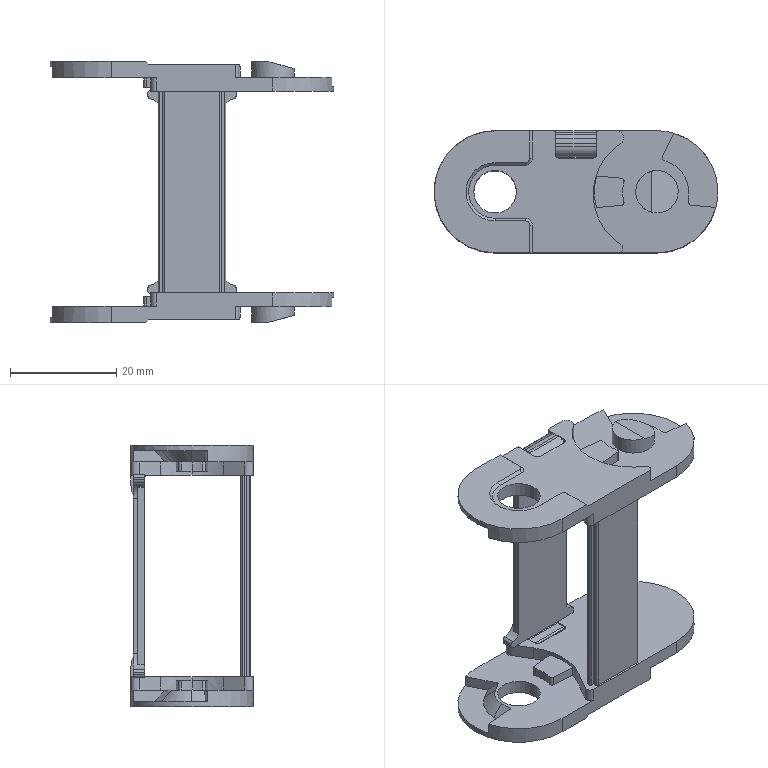Part | SolidWorks | features BaseBody 1 | 1 solid | 246 faces | box 53.492 x 23 x 49.2 mm | volume 8720 mm3 | cylinder 118 | plane 114 | spline 8 | cone 6 | commonest cylinder face diameters 1 x26 0.6 x15 2 x9 1.2 x6 2.4 x6 8 x6